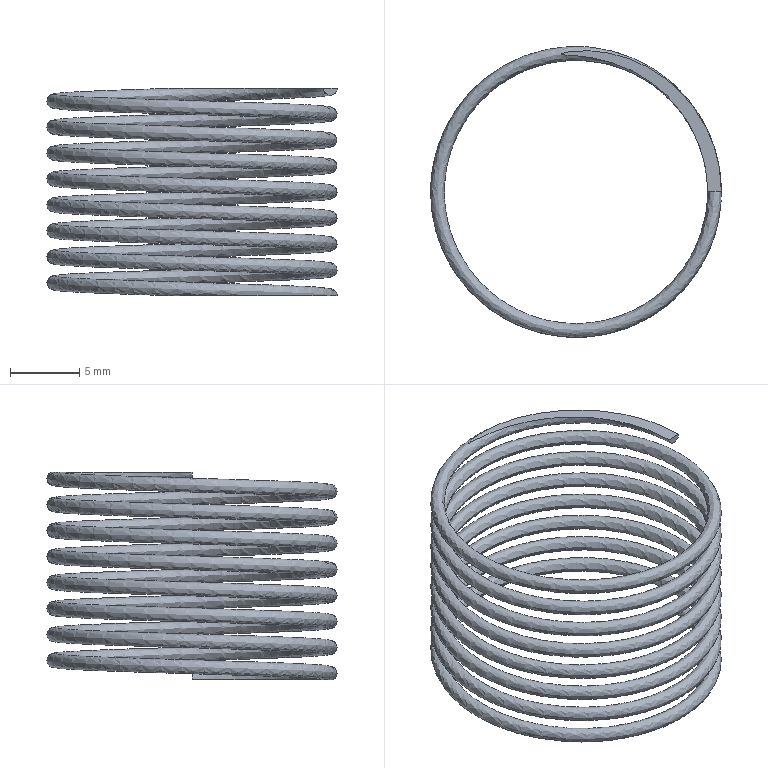Part | STEP file | tanhuang | 1 solid | 5 faces | volume 381.944 mm3 | plane 4 | spline 1